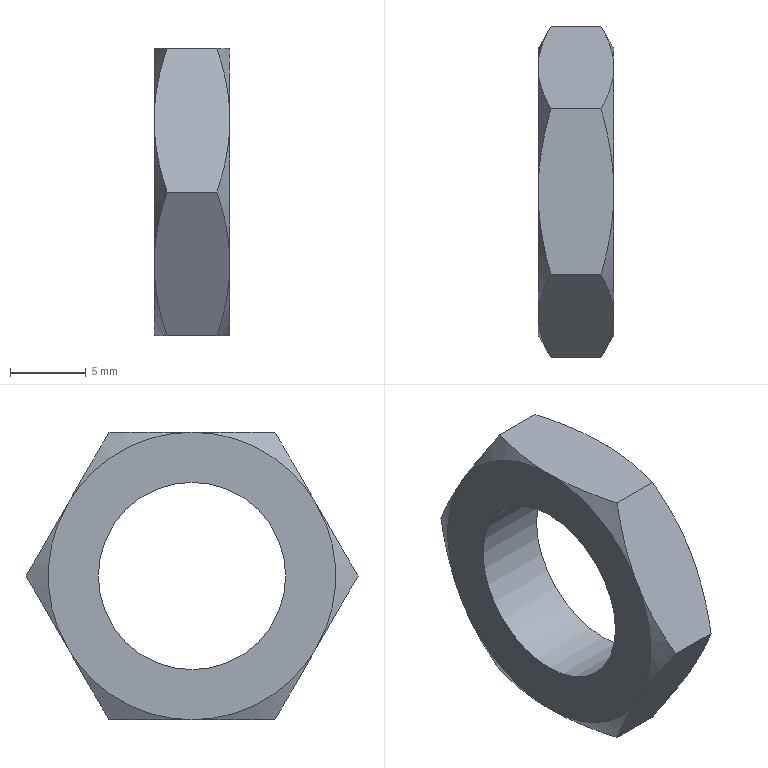Part | NX | features NAT_5003_019_C-AC1412S 2 | 1 solid | 21 faces | box 5 x 21.939 x 19 mm | volume 946.478 mm3 | cone 12 | plane 8 | cylinder 1 | commonest cylinder face diameters 12.376 x1
STEP:
#1=CARTESIAN_POINT('',(56.752,-131.515,-232.5));
#2=VERTEX_POINT('',#1);
#3=CARTESIAN_POINT('',(57.6,-128.773,-227.75));
#4=VERTEX_POINT('',#3);
#5=CARTESIAN_POINT('',(56.752,-131.515,-232.5));
#6=CARTESIAN_POINT('',(57.27,-130.618,-230.946));
#7=CARTESIAN_POINT('',(57.6,-129.707,-229.369));
#8=CARTESIAN_POINT('',(57.6,-128.773,-227.75));
#9=B_SPLINE_CURVE_WITH_KNOTS('',3,(#5,#6,#7,#8),.UNSPECIFIED.,.F.,.F.,(4,4),(0.000000238,0.00555),.UNSPECIFIED.);
#10=EDGE_CURVE('',#2,#4,#9,.T.);
#11=ORIENTED_EDGE('',*,*,#10,.F.);
#12=CARTESIAN_POINT('',(53.449,-131.515,-232.5));
#13=VERTEX_POINT('',#12);
#14=CARTESIAN_POINT('',(57.6,-131.515,-232.5));
#15=DIRECTION('',(-1.,0.,0.));
#16=VECTOR('',#15,1000.);
#17=LINE('',#14,#16);
#18=EDGE_CURVE('',#2,#13,#17,.T.);
#19=ORIENTED_EDGE('',*,*,#18,.T.);
#20=CARTESIAN_POINT('',(52.6,-128.773,-227.75));
#21=VERTEX_POINT('',#20);
#22=CARTESIAN_POINT('',(52.6,-128.773,-227.75));
#23=CARTESIAN_POINT('',(52.6,-129.704,-229.362));
#24=CARTESIAN_POINT('',(52.932,-130.62,-230.95));
#25=CARTESIAN_POINT('',(53.449,-131.515,-232.5));
#26=B_SPLINE_CURVE_WITH_KNOTS('',3,(#22,#23,#24,#25),.UNSPECIFIED.,.F.,.F.,(4,4),(0.00555,0.01108),.UNSPECIFIED.);
#27=EDGE_CURVE('',#21,#13,#26,.T.);
#28=ORIENTED_EDGE('',*,*,#27,.F.);
#29=CARTESIAN_POINT('',(53.449,-126.03,-223.));
#30=VERTEX_POINT('',#29);
#31=CARTESIAN_POINT('',(53.449,-126.03,-223.));
#32=CARTESIAN_POINT('',(52.931,-126.928,-224.554));
#33=CARTESIAN_POINT('',(52.6,-127.838,-226.131));
#34=CARTESIAN_POINT('',(52.6,-128.773,-227.75));
#35=B_SPLINE_CURVE_WITH_KNOTS('',3,(#31,#32,#33,#34),.UNSPECIFIED.,.F.,.F.,(4,4),(0.000000238,0.00555),.UNSPECIFIED.);
#36=EDGE_CURVE('',#30,#21,#35,.T.);
#37=ORIENTED_EDGE('',*,*,#36,.F.);
#38=CARTESIAN_POINT('',(56.752,-126.03,-223.));
#39=VERTEX_POINT('',#38);
#40=CARTESIAN_POINT('',(57.6,-126.03,-223.));
#41=DIRECTION('',(-1.,0.,0.));
#42=VECTOR('',#41,1000.);
#43=LINE('',#40,#42);
#44=EDGE_CURVE('',#39,#30,#43,.T.);
#45=ORIENTED_EDGE('',*,*,#44,.F.);
#46=CARTESIAN_POINT('',(57.6,-128.773,-227.75));
#47=CARTESIAN_POINT('',(57.6,-127.842,-226.138));
#48=CARTESIAN_POINT('',(57.269,-126.925,-224.55));
#49=CARTESIAN_POINT('',(56.752,-126.03,-223.));
#50=B_SPLINE_CURVE_WITH_KNOTS('',3,(#46,#47,#48,#49),.UNSPECIFIED.,.F.,.F.,(4,4),(0.00555,0.01108),.UNSPECIFIED.);
#51=EDGE_CURVE('',#4,#39,#50,.T.);
#52=ORIENTED_EDGE('',*,*,#51,.F.);
#53=EDGE_LOOP('',(#11,#19,#28,#37,#45,#52));
#54=FACE_BOUND('',#53,.T.);
#55=CARTESIAN_POINT('',(57.6,-131.515,-232.5));
#56=DIRECTION('',(0.,-0.866,0.5));
#57=DIRECTION('',(0.,-0.5,-0.866));
#58=AXIS2_PLACEMENT_3D('',#55,#56,#57);
#59=PLANE('',#58);
#60=ADVANCED_FACE('',(#54),#59,.F.);
#61=CARTESIAN_POINT('',(57.6,-128.773,-218.25));
#62=VERTEX_POINT('',#61);
#63=CARTESIAN_POINT('',(56.752,-126.03,-223.));
#64=CARTESIAN_POINT('',(57.27,-126.928,-221.446));
#65=CARTESIAN_POINT('',(57.6,-127.838,-219.869));
#66=CARTESIAN_POINT('',(57.6,-128.773,-218.25));
#67=B_SPLINE_CURVE_WITH_KNOTS('',3,(#63,#64,#65,#66),.UNSPECIFIED.,.F.,.F.,(4,4),(0.000000238,0.00555),.UNSPECIFIED.);
#68=EDGE_CURVE('',#39,#62,#67,.T.);
#69=ORIENTED_EDGE('',*,*,#68,.F.);
#70=ORIENTED_EDGE('',*,*,#44,.T.);
#71=CARTESIAN_POINT('',(52.6,-128.773,-218.25));
#72=VERTEX_POINT('',#71);
#73=CARTESIAN_POINT('',(52.6,-128.773,-218.25));
#74=CARTESIAN_POINT('',(52.6,-127.842,-219.862));
#75=CARTESIAN_POINT('',(52.932,-126.925,-221.45));
#76=CARTESIAN_POINT('',(53.449,-126.03,-223.));
#77=B_SPLINE_CURVE_WITH_KNOTS('',3,(#73,#74,#75,#76),.UNSPECIFIED.,.F.,.F.,(4,4),(0.00555,0.01108),.UNSPECIFIED.);
#78=EDGE_CURVE('',#72,#30,#77,.T.);
#79=ORIENTED_EDGE('',*,*,#78,.F.);
#80=CARTESIAN_POINT('',(53.449,-131.515,-213.5));
#81=VERTEX_POINT('',#80);
#82=CARTESIAN_POINT('',(53.449,-131.515,-213.5));
#83=CARTESIAN_POINT('',(52.931,-130.618,-215.054));
#84=CARTESIAN_POINT('',(52.6,-129.707,-216.631));
#85=CARTESIAN_POINT('',(52.6,-128.773,-218.25));
#86=B_SPLINE_CURVE_WITH_KNOTS('',3,(#82,#83,#84,#85),.UNSPECIFIED.,.F.,.F.,(4,4),(0.000000238,0.00555),.UNSPECIFIED.);
#87=EDGE_CURVE('',#81,#72,#86,.T.);
#88=ORIENTED_EDGE('',*,*,#87,.F.);
#89=CARTESIAN_POINT('',(56.752,-131.515,-213.5));
#90=VERTEX_POINT('',#89);
#91=CARTESIAN_POINT('',(57.6,-131.515,-213.5));
#92=DIRECTION('',(-1.,0.,0.));
#93=VECTOR('',#92,1000.);
#94=LINE('',#91,#93);
#95=EDGE_CURVE('',#90,#81,#94,.T.);
#96=ORIENTED_EDGE('',*,*,#95,.F.);
#97=CARTESIAN_POINT('',(57.6,-128.773,-218.25));
#98=CARTESIAN_POINT('',(57.6,-129.704,-216.638));
#99=CARTESIAN_POINT('',(57.269,-130.62,-215.05));
#100=CARTESIAN_POINT('',(56.752,-131.515,-213.5));
#101=B_SPLINE_CURVE_WITH_KNOTS('',3,(#97,#98,#99,#100),.UNSPECIFIED.,.F.,.F.,(4,4),(0.00555,0.01108),.UNSPECIFIED.);
#102=EDGE_CURVE('',#62,#90,#101,.T.);
#103=ORIENTED_EDGE('',*,*,#102,.F.);
#104=EDGE_LOOP('',(#69,#70,#79,#88,#96,#103));
#105=FACE_BOUND('',#104,.T.);
#106=CARTESIAN_POINT('',(57.6,-126.03,-223.));
#107=DIRECTION('',(0.,-0.866,-0.5));
#108=DIRECTION('',(0.,0.5,-0.866));
#109=AXIS2_PLACEMENT_3D('',#106,#107,#108);
#110=PLANE('',#109);
#111=ADVANCED_FACE('',(#105),#110,.F.);
#112=CARTESIAN_POINT('',(57.6,-137.,-213.5));
#113=VERTEX_POINT('',#112);
#114=CARTESIAN_POINT('',(56.752,-131.515,-213.5));
#115=CARTESIAN_POINT('',(57.267,-133.301,-213.5));
#116=CARTESIAN_POINT('',(57.6,-135.145,-213.5));
#117=CARTESIAN_POINT('',(57.6,-137.,-213.5));
#118=B_SPLINE_CURVE_WITH_KNOTS('',3,(#114,#115,#116,#117),.UNSPECIFIED.,.F.,.F.,(4,4),(0.01001,0.01556),.UNSPECIFIED.);
#119=EDGE_CURVE('',#90,#113,#118,.T.);
#120=ORIENTED_EDGE('',*,*,#119,.F.);
#121=ORIENTED_EDGE('',*,*,#95,.T.);
#122=CARTESIAN_POINT('',(52.6,-137.,-213.5));
#123=VERTEX_POINT('',#122);
#124=CARTESIAN_POINT('',(53.449,-131.515,-213.5));
#125=CARTESIAN_POINT('',(52.934,-133.301,-213.5));
#126=CARTESIAN_POINT('',(52.6,-135.145,-213.5));
#127=CARTESIAN_POINT('',(52.6,-137.,-213.5));
#128=B_SPLINE_CURVE_WITH_KNOTS('',3,(#124,#125,#126,#127),.UNSPECIFIED.,.F.,.F.,(4,4),(0.01001,0.01556),.UNSPECIFIED.);
#129=EDGE_CURVE('',#123,#81,#128,.F.);
#130=ORIENTED_EDGE('',*,*,#129,.F.);
#131=CARTESIAN_POINT('',(53.449,-142.485,-213.5));
#132=VERTEX_POINT('',#131);
#133=CARTESIAN_POINT('',(52.6,-137.,-213.5));
#134=CARTESIAN_POINT('',(52.6,-138.856,-213.5));
#135=CARTESIAN_POINT('',(52.937,-140.711,-213.5));
#136=CARTESIAN_POINT('',(53.449,-142.485,-213.5));
#137=B_SPLINE_CURVE_WITH_KNOTS('',3,(#133,#134,#135,#136),.UNSPECIFIED.,.F.,.F.,(4,4),(0.01556,0.02112),.UNSPECIFIED.);
#138=EDGE_CURVE('',#132,#123,#137,.F.);
#139=ORIENTED_EDGE('',*,*,#138,.F.);
#140=CARTESIAN_POINT('',(56.752,-142.485,-213.5));
#141=VERTEX_POINT('',#140);
#142=CARTESIAN_POINT('',(57.6,-142.485,-213.5));
#143=DIRECTION('',(-1.,0.,0.));
#144=VECTOR('',#143,1000.);
#145=LINE('',#142,#144);
#146=EDGE_CURVE('',#141,#132,#145,.T.);
#147=ORIENTED_EDGE('',*,*,#146,.F.);
#148=CARTESIAN_POINT('',(57.6,-137.,-213.5));
#149=CARTESIAN_POINT('',(57.6,-138.856,-213.5));
#150=CARTESIAN_POINT('',(57.264,-140.711,-213.5));
#151=CARTESIAN_POINT('',(56.752,-142.485,-213.5));
#152=B_SPLINE_CURVE_WITH_KNOTS('',3,(#148,#149,#150,#151),.UNSPECIFIED.,.F.,.F.,(4,4),(0.01556,0.02112),.UNSPECIFIED.);
#153=EDGE_CURVE('',#113,#141,#152,.T.);
#154=ORIENTED_EDGE('',*,*,#153,.F.);
#155=EDGE_LOOP('',(#120,#121,#130,#139,#147,#154));
#156=FACE_BOUND('',#155,.T.);
#157=CARTESIAN_POINT('',(57.6,-131.515,-213.5));
#158=DIRECTION('',(0.,0.,-1.));
#159=DIRECTION('',(0.,1.,0.));
#160=AXIS2_PLACEMENT_3D('',#157,#158,#159);
#161=PLANE('',#160);
#162=ADVANCED_FACE('',(#156),#161,.F.);
#163=CARTESIAN_POINT('',(57.6,-145.227,-218.25));
#164=VERTEX_POINT('',#163);
#165=CARTESIAN_POINT('',(56.752,-142.485,-213.5));
#166=CARTESIAN_POINT('',(57.27,-143.382,-215.054));
#167=CARTESIAN_POINT('',(57.6,-144.293,-216.631));
#168=CARTESIAN_POINT('',(57.6,-145.227,-218.25));
#169=B_SPLINE_CURVE_WITH_KNOTS('',3,(#165,#166,#167,#168),.UNSPECIFIED.,.F.,.F.,(4,4),(0.000000238,0.00555),.UNSPECIFIED.);
#170=EDGE_CURVE('',#141,#164,#169,.T.);
#171=ORIENTED_EDGE('',*,*,#170,.F.);
#172=ORIENTED_EDGE('',*,*,#146,.T.);
#173=CARTESIAN_POINT('',(52.6,-145.227,-218.25));
#174=VERTEX_POINT('',#173);
#175=CARTESIAN_POINT('',(52.6,-145.227,-218.25));
#176=CARTESIAN_POINT('',(52.6,-144.296,-216.638));
#177=CARTESIAN_POINT('',(52.932,-143.38,-215.05));
#178=CARTESIAN_POINT('',(53.449,-142.485,-213.5));
#179=B_SPLINE_CURVE_WITH_KNOTS('',3,(#175,#176,#177,#178),.UNSPECIFIED.,.F.,.F.,(4,4),(0.00555,0.01108),.UNSPECIFIED.);
#180=EDGE_CURVE('',#174,#132,#179,.T.);
#181=ORIENTED_EDGE('',*,*,#180,.F.);
#182=CARTESIAN_POINT('',(53.449,-147.97,-223.));
#183=VERTEX_POINT('',#182);
#184=CARTESIAN_POINT('',(53.449,-147.97,-223.));
#185=CARTESIAN_POINT('',(52.931,-147.072,-221.446));
#186=CARTESIAN_POINT('',(52.6,-146.162,-219.869));
#187=CARTESIAN_POINT('',(52.6,-145.227,-218.25));
#188=B_SPLINE_CURVE_WITH_KNOTS('',3,(#184,#185,#186,#187),.UNSPECIFIED.,.F.,.F.,(4,4),(0.000000238,0.00555),.UNSPECIFIED.);
#189=EDGE_CURVE('',#183,#174,#188,.T.);
#190=ORIENTED_EDGE('',*,*,#189,.F.);
#191=CARTESIAN_POINT('',(56.752,-147.97,-223.));
#192=VERTEX_POINT('',#191);
#193=CARTESIAN_POINT('',(57.6,-147.97,-223.));
#194=DIRECTION('',(-1.,0.,0.));
#195=VECTOR('',#194,1000.);
#196=LINE('',#193,#195);
#197=EDGE_CURVE('',#192,#183,#196,.T.);
#198=ORIENTED_EDGE('',*,*,#197,.F.);
#199=CARTESIAN_POINT('',(57.6,-145.227,-218.25));
#200=CARTESIAN_POINT('',(57.6,-146.158,-219.862));
#201=CARTESIAN_POINT('',(57.269,-147.075,-221.45));
#202=CARTESIAN_POINT('',(56.752,-147.97,-223.));
#203=B_SPLINE_CURVE_WITH_KNOTS('',3,(#199,#200,#201,#202),.UNSPECIFIED.,.F.,.F.,(4,4),(0.00555,0.01108),.UNSPECIFIED.);
#204=EDGE_CURVE('',#164,#192,#203,.T.);
#205=ORIENTED_EDGE('',*,*,#204,.F.);
#206=EDGE_LOOP('',(#171,#172,#181,#190,#198,#205));
#207=FACE_BOUND('',#206,.T.);
#208=CARTESIAN_POINT('',(57.6,-142.485,-213.5));
#209=DIRECTION('',(0.,0.866,-0.5));
#210=DIRECTION('',(0.,0.5,0.866));
#211=AXIS2_PLACEMENT_3D('',#208,#209,#210);
#212=PLANE('',#211);
#213=ADVANCED_FACE('',(#207),#212,.F.);
#214=CARTESIAN_POINT('',(57.6,-145.227,-227.75));
#215=VERTEX_POINT('',#214);
#216=CARTESIAN_POINT('',(56.752,-147.97,-223.));
#217=CARTESIAN_POINT('',(57.27,-147.072,-224.554));
#218=CARTESIAN_POINT('',(57.6,-146.162,-226.131));
#219=CARTESIAN_POINT('',(57.6,-145.227,-227.75));
#220=B_SPLINE_CURVE_WITH_KNOTS('',3,(#216,#217,#218,#219),.UNSPECIFIED.,.F.,.F.,(4,4),(0.000000238,0.00555),.UNSPECIFIED.);
#221=EDGE_CURVE('',#192,#215,#220,.T.);
#222=ORIENTED_EDGE('',*,*,#221,.F.);
#223=ORIENTED_EDGE('',*,*,#197,.T.);
#224=CARTESIAN_POINT('',(52.6,-145.227,-227.75));
#225=VERTEX_POINT('',#224);
#226=CARTESIAN_POINT('',(52.6,-145.227,-227.75));
#227=CARTESIAN_POINT('',(52.6,-146.158,-226.138));
#228=CARTESIAN_POINT('',(52.932,-147.075,-224.55));
#229=CARTESIAN_POINT('',(53.449,-147.97,-223.));
#230=B_SPLINE_CURVE_WITH_KNOTS('',3,(#226,#227,#228,#229),.UNSPECIFIED.,.F.,.F.,(4,4),(0.00555,0.01108),.UNSPECIFIED.);
#231=EDGE_CURVE('',#225,#183,#230,.T.);
#232=ORIENTED_EDGE('',*,*,#231,.F.);
#233=CARTESIAN_POINT('',(53.449,-142.485,-232.5));
#234=VERTEX_POINT('',#233);
#235=CARTESIAN_POINT('',(53.449,-142.485,-232.5));
#236=CARTESIAN_POINT('',(52.931,-143.382,-230.946));
#237=CARTESIAN_POINT('',(52.6,-144.293,-229.369));
#238=CARTESIAN_POINT('',(52.6,-145.227,-227.75));
#239=B_SPLINE_CURVE_WITH_KNOTS('',3,(#235,#236,#237,#238),.UNSPECIFIED.,.F.,.F.,(4,4),(0.000000238,0.00555),.UNSPECIFIED.);
#240=EDGE_CURVE('',#234,#225,#239,.T.);
#241=ORIENTED_EDGE('',*,*,#240,.F.);
#242=CARTESIAN_POINT('',(56.752,-142.485,-232.5));
#243=VERTEX_POINT('',#242);
#244=CARTESIAN_POINT('',(57.6,-142.485,-232.5));
#245=DIRECTION('',(-1.,0.,0.));
#246=VECTOR('',#245,1000.);
#247=LINE('',#244,#246);
#248=EDGE_CURVE('',#243,#234,#247,.T.);
#249=ORIENTED_EDGE('',*,*,#248,.F.);
#250=CARTESIAN_POINT('',(57.6,-145.227,-227.75));
#251=CARTESIAN_POINT('',(57.6,-144.296,-229.362));
#252=CARTESIAN_POINT('',(57.269,-143.38,-230.95));
#253=CARTESIAN_POINT('',(56.752,-142.485,-232.5));
#254=B_SPLINE_CURVE_WITH_KNOTS('',3,(#250,#251,#252,#253),.UNSPECIFIED.,.F.,.F.,(4,4),(0.00555,0.01108),.UNSPECIFIED.);
#255=EDGE_CURVE('',#215,#243,#254,.T.);
#256=ORIENTED_EDGE('',*,*,#255,.F.);
#257=EDGE_LOOP('',(#222,#223,#232,#241,#249,#256));
#258=FACE_BOUND('',#257,.T.);
#259=CARTESIAN_POINT('',(57.6,-147.97,-223.));
#260=DIRECTION('',(0.,0.866,0.5));
#261=DIRECTION('',(0.,-0.5,0.866));
#262=AXIS2_PLACEMENT_3D('',#259,#260,#261);
#263=PLANE('',#262);
#264=ADVANCED_FACE('',(#258),#263,.F.);
#265=CARTESIAN_POINT('',(57.6,-137.,-232.5));
#266=VERTEX_POINT('',#265);
#267=CARTESIAN_POINT('',(57.6,-137.,-232.5));
#268=CARTESIAN_POINT('',(57.6,-138.856,-232.5));
#269=CARTESIAN_POINT('',(57.264,-140.711,-232.5));
#270=CARTESIAN_POINT('',(56.752,-142.485,-232.5));
#271=B_SPLINE_CURVE_WITH_KNOTS('',3,(#267,#268,#269,#270),.UNSPECIFIED.,.F.,.F.,(4,4),(0.01556,0.02112),.UNSPECIFIED.);
#272=EDGE_CURVE('',#243,#266,#271,.F.);
#273=ORIENTED_EDGE('',*,*,#272,.F.);
#274=ORIENTED_EDGE('',*,*,#248,.T.);
#275=CARTESIAN_POINT('',(52.6,-137.,-232.5));
#276=VERTEX_POINT('',#275);
#277=CARTESIAN_POINT('',(52.6,-137.,-232.5));
#278=CARTESIAN_POINT('',(52.6,-138.856,-232.5));
#279=CARTESIAN_POINT('',(52.937,-140.711,-232.5));
#280=CARTESIAN_POINT('',(53.449,-142.485,-232.5));
#281=B_SPLINE_CURVE_WITH_KNOTS('',3,(#277,#278,#279,#280),.UNSPECIFIED.,.F.,.F.,(4,4),(0.01556,0.02112),.UNSPECIFIED.);
#282=EDGE_CURVE('',#276,#234,#281,.T.);
#283=ORIENTED_EDGE('',*,*,#282,.F.);
#284=CARTESIAN_POINT('',(53.449,-131.515,-232.5));
#285=CARTESIAN_POINT('',(52.934,-133.301,-232.5));
#286=CARTESIAN_POINT('',(52.6,-135.145,-232.5));
#287=CARTESIAN_POINT('',(52.6,-137.,-232.5));
#288=B_SPLINE_CURVE_WITH_KNOTS('',3,(#284,#285,#286,#287),.UNSPECIFIED.,.F.,.F.,(4,4),(0.01001,0.01556),.UNSPECIFIED.);
#289=EDGE_CURVE('',#13,#276,#288,.T.);
#290=ORIENTED_EDGE('',*,*,#289,.F.);
#291=ORIENTED_EDGE('',*,*,#18,.F.);
#292=CARTESIAN_POINT('',(56.752,-131.515,-232.5));
#293=CARTESIAN_POINT('',(57.267,-133.301,-232.5));
#294=CARTESIAN_POINT('',(57.6,-135.145,-232.5));
#295=CARTESIAN_POINT('',(57.6,-137.,-232.5));
#296=B_SPLINE_CURVE_WITH_KNOTS('',3,(#292,#293,#294,#295),.UNSPECIFIED.,.F.,.F.,(4,4),(0.01001,0.01556),.UNSPECIFIED.);
#297=EDGE_CURVE('',#266,#2,#296,.F.);
#298=ORIENTED_EDGE('',*,*,#297,.F.);
#299=EDGE_LOOP('',(#273,#274,#283,#290,#291,#298));
#300=FACE_BOUND('',#299,.T.);
#301=CARTESIAN_POINT('',(57.6,-142.485,-232.5));
#302=DIRECTION('',(0.,0.,1.));
#303=DIRECTION('',(0.,-1.,0.));
#304=AXIS2_PLACEMENT_3D('',#301,#302,#303);
#305=PLANE('',#304);
#306=ADVANCED_FACE('',(#300),#305,.F.);
#307=CARTESIAN_POINT('',(57.6,-130.812,-223.));
#308=VERTEX_POINT('',#307);
#309=CARTESIAN_POINT('',(57.6,-137.,-223.));
#310=DIRECTION('',(1.,0.,0.));
#311=DIRECTION('',(0.,1.,0.));
#312=AXIS2_PLACEMENT_3D('',#309,#310,#311);
#313=CIRCLE('',#312,6.188);
#314=EDGE_CURVE('',#308,#308,#313,.T.);
#315=ORIENTED_EDGE('',*,*,#314,.F.);
#316=EDGE_LOOP('',(#315));
#317=FACE_BOUND('',#316,.T.);
#318=CARTESIAN_POINT('',(57.6,-137.,-223.));
#319=DIRECTION('',(1.,0.,0.));
#320=DIRECTION('',(0.,1.,0.));
#321=AXIS2_PLACEMENT_3D('',#318,#319,#320);
#322=CIRCLE('',#321,9.5);
#323=EDGE_CURVE('',#4,#62,#322,.T.);
#324=ORIENTED_EDGE('',*,*,#323,.T.);
#325=CARTESIAN_POINT('',(57.6,-137.,-223.));
#326=DIRECTION('',(1.,0.,0.));
#327=DIRECTION('',(0.,1.,0.));
#328=AXIS2_PLACEMENT_3D('',#325,#326,#327);
#329=CIRCLE('',#328,9.5);
#330=EDGE_CURVE('',#62,#113,#329,.T.);
#331=ORIENTED_EDGE('',*,*,#330,.T.);
#332=CARTESIAN_POINT('',(57.6,-137.,-223.));
#333=DIRECTION('',(-1.,0.,0.));
#334=DIRECTION('',(0.,-1.,0.));
#335=AXIS2_PLACEMENT_3D('',#332,#333,#334);
#336=CIRCLE('',#335,9.5);
#337=EDGE_CURVE('',#164,#113,#336,.T.);
#338=ORIENTED_EDGE('',*,*,#337,.F.);
#339=CARTESIAN_POINT('',(57.6,-137.,-223.));
#340=DIRECTION('',(1.,0.,0.));
#341=DIRECTION('',(0.,1.,0.));
#342=AXIS2_PLACEMENT_3D('',#339,#340,#341);
#343=CIRCLE('',#342,9.5);
#344=EDGE_CURVE('',#164,#215,#343,.T.);
#345=ORIENTED_EDGE('',*,*,#344,.T.);
#346=CARTESIAN_POINT('',(57.6,-137.,-223.));
#347=DIRECTION('',(1.,0.,0.));
#348=DIRECTION('',(0.,1.,0.));
#349=AXIS2_PLACEMENT_3D('',#346,#347,#348);
#350=CIRCLE('',#349,9.5);
#351=EDGE_CURVE('',#215,#266,#350,.T.);
#352=ORIENTED_EDGE('',*,*,#351,.T.);
#353=CARTESIAN_POINT('',(57.6,-137.,-223.));
#354=DIRECTION('',(1.,0.,0.));
#355=DIRECTION('',(0.,1.,0.));
#356=AXIS2_PLACEMENT_3D('',#353,#354,#355);
#357=CIRCLE('',#356,9.5);
#358=EDGE_CURVE('',#266,#4,#357,.T.);
#359=ORIENTED_EDGE('',*,*,#358,.T.);
#360=EDGE_LOOP('',(#324,#331,#338,#345,#352,#359));
#361=FACE_BOUND('',#360,.T.);
#362=CARTESIAN_POINT('',(57.6,-137.,-223.));
#363=DIRECTION('',(1.,0.,0.));
#364=DIRECTION('',(0.,1.,0.));
#365=AXIS2_PLACEMENT_3D('',#362,#363,#364);
#366=PLANE('',#365);
#367=ADVANCED_FACE('',(#317,#361),#366,.T.);
#368=CARTESIAN_POINT('',(52.6,-130.812,-223.));
#369=VERTEX_POINT('',#368);
#370=CARTESIAN_POINT('',(52.6,-137.,-223.));
#371=DIRECTION('',(1.,0.,0.));
#372=DIRECTION('',(0.,1.,0.));
#373=AXIS2_PLACEMENT_3D('',#370,#371,#372);
#374=CIRCLE('',#373,6.188);
#375=EDGE_CURVE('',#369,#369,#374,.T.);
#376=ORIENTED_EDGE('',*,*,#375,.T.);
#377=EDGE_LOOP('',(#376));
#378=FACE_BOUND('',#377,.T.);
#379=CARTESIAN_POINT('',(52.6,-137.,-223.));
#380=DIRECTION('',(1.,0.,0.));
#381=DIRECTION('',(0.,1.,0.));
#382=AXIS2_PLACEMENT_3D('',#379,#380,#381);
#383=CIRCLE('',#382,9.5);
#384=EDGE_CURVE('',#72,#123,#383,.T.);
#385=ORIENTED_EDGE('',*,*,#384,.F.);
#386=CARTESIAN_POINT('',(52.6,-137.,-223.));
#387=DIRECTION('',(1.,0.,0.));
#388=DIRECTION('',(0.,1.,0.));
#389=AXIS2_PLACEMENT_3D('',#386,#387,#388);
#390=CIRCLE('',#389,9.5);
#391=EDGE_CURVE('',#21,#72,#390,.T.);
#392=ORIENTED_EDGE('',*,*,#391,.F.);
#393=CARTESIAN_POINT('',(52.6,-137.,-223.));
#394=DIRECTION('',(1.,0.,0.));
#395=DIRECTION('',(0.,1.,0.));
#396=AXIS2_PLACEMENT_3D('',#393,#394,#395);
#397=CIRCLE('',#396,9.5);
#398=EDGE_CURVE('',#276,#21,#397,.T.);
#399=ORIENTED_EDGE('',*,*,#398,.F.);
#400=CARTESIAN_POINT('',(52.6,-137.,-223.));
#401=DIRECTION('',(1.,0.,0.));
#402=DIRECTION('',(0.,1.,0.));
#403=AXIS2_PLACEMENT_3D('',#400,#401,#402);
#404=CIRCLE('',#403,9.5);
#405=EDGE_CURVE('',#225,#276,#404,.T.);
#406=ORIENTED_EDGE('',*,*,#405,.F.);
#407=CARTESIAN_POINT('',(52.6,-137.,-223.));
#408=DIRECTION('',(1.,0.,0.));
#409=DIRECTION('',(0.,1.,0.));
#410=AXIS2_PLACEMENT_3D('',#407,#408,#409);
#411=CIRCLE('',#410,9.5);
#412=EDGE_CURVE('',#174,#225,#411,.T.);
#413=ORIENTED_EDGE('',*,*,#412,.F.);
#414=CARTESIAN_POINT('',(52.6,-137.,-223.));
#415=DIRECTION('',(-1.,0.,0.));
#416=DIRECTION('',(0.,-1.,0.));
#417=AXIS2_PLACEMENT_3D('',#414,#415,#416);
#418=CIRCLE('',#417,9.5);
#419=EDGE_CURVE('',#174,#123,#418,.T.);
#420=ORIENTED_EDGE('',*,*,#419,.T.);
#421=EDGE_LOOP('',(#385,#392,#399,#406,#413,#420));
#422=FACE_BOUND('',#421,.T.);
#423=CARTESIAN_POINT('',(52.6,-137.,-223.));
#424=DIRECTION('',(1.,0.,0.));
#425=DIRECTION('',(0.,1.,0.));
#426=AXIS2_PLACEMENT_3D('',#423,#424,#425);
#427=PLANE('',#426);
#428=ADVANCED_FACE('',(#378,#422),#427,.F.);
#429=ORIENTED_EDGE('',*,*,#375,.F.);
#430=EDGE_LOOP('',(#429));
#431=FACE_BOUND('',#430,.T.);
#432=ORIENTED_EDGE('',*,*,#314,.T.);
#433=EDGE_LOOP('',(#432));
#434=FACE_BOUND('',#433,.T.);
#435=CARTESIAN_POINT('',(57.6,-137.,-223.));
#436=DIRECTION('',(1.,0.,0.));
#437=DIRECTION('',(0.,1.,0.));
#438=AXIS2_PLACEMENT_3D('',#435,#436,#437);
#439=CYLINDRICAL_SURFACE('',#438,6.188);
#440=ADVANCED_FACE('',(#431,#434),#439,.F.);
#441=ORIENTED_EDGE('',*,*,#78,.T.);
#442=ORIENTED_EDGE('',*,*,#36,.T.);
#443=ORIENTED_EDGE('',*,*,#391,.T.);
#444=EDGE_LOOP('',(#441,#442,#443));
#445=FACE_BOUND('',#444,.T.);
#446=CARTESIAN_POINT('',(52.6,-137.,-223.));
#447=DIRECTION('',(1.,0.,0.));
#448=DIRECTION('',(0.,1.,0.));
#449=AXIS2_PLACEMENT_3D('',#446,#447,#448);
#450=CONICAL_SURFACE('',#449,9.5,1.047);
#451=ADVANCED_FACE('',(#445),#450,.T.);
#452=ORIENTED_EDGE('',*,*,#27,.T.);
#453=ORIENTED_EDGE('',*,*,#289,.T.);
#454=ORIENTED_EDGE('',*,*,#398,.T.);
#455=EDGE_LOOP('',(#452,#453,#454));
#456=FACE_BOUND('',#455,.T.);
#457=CARTESIAN_POINT('',(52.6,-137.,-223.));
#458=DIRECTION('',(1.,0.,0.));
#459=DIRECTION('',(0.,1.,0.));
#460=AXIS2_PLACEMENT_3D('',#457,#458,#459);
#461=CONICAL_SURFACE('',#460,9.5,1.047);
#462=ADVANCED_FACE('',(#456),#461,.T.);
#463=ORIENTED_EDGE('',*,*,#240,.T.);
#464=ORIENTED_EDGE('',*,*,#405,.T.);
#465=ORIENTED_EDGE('',*,*,#282,.T.);
#466=EDGE_LOOP('',(#463,#464,#465));
#467=FACE_BOUND('',#466,.T.);
#468=CARTESIAN_POINT('',(52.6,-137.,-223.));
#469=DIRECTION('',(1.,0.,0.));
#470=DIRECTION('',(0.,1.,0.));
#471=AXIS2_PLACEMENT_3D('',#468,#469,#470);
#472=CONICAL_SURFACE('',#471,9.5,1.047);
#473=ADVANCED_FACE('',(#467),#472,.T.);
#474=ORIENTED_EDGE('',*,*,#189,.T.);
#475=ORIENTED_EDGE('',*,*,#412,.T.);
#476=ORIENTED_EDGE('',*,*,#231,.T.);
#477=EDGE_LOOP('',(#474,#475,#476));
#478=FACE_BOUND('',#477,.T.);
#479=CARTESIAN_POINT('',(52.6,-137.,-223.));
#480=DIRECTION('',(1.,0.,0.));
#481=DIRECTION('',(0.,1.,0.));
#482=AXIS2_PLACEMENT_3D('',#479,#480,#481);
#483=CONICAL_SURFACE('',#482,9.5,1.047);
#484=ADVANCED_FACE('',(#478),#483,.T.);
#485=ORIENTED_EDGE('',*,*,#138,.T.);
#486=ORIENTED_EDGE('',*,*,#419,.F.);
#487=ORIENTED_EDGE('',*,*,#180,.T.);
#488=EDGE_LOOP('',(#485,#486,#487));
#489=FACE_BOUND('',#488,.T.);
#490=CARTESIAN_POINT('',(52.6,-137.,-223.));
#491=DIRECTION('',(1.,0.,0.));
#492=DIRECTION('',(0.,1.,0.));
#493=AXIS2_PLACEMENT_3D('',#490,#491,#492);
#494=CONICAL_SURFACE('',#493,9.5,1.047);
#495=ADVANCED_FACE('',(#489),#494,.T.);
#496=ORIENTED_EDGE('',*,*,#129,.T.);
#497=ORIENTED_EDGE('',*,*,#87,.T.);
#498=ORIENTED_EDGE('',*,*,#384,.T.);
#499=EDGE_LOOP('',(#496,#497,#498));
#500=FACE_BOUND('',#499,.T.);
#501=CARTESIAN_POINT('',(52.6,-137.,-223.));
#502=DIRECTION('',(1.,0.,0.));
#503=DIRECTION('',(0.,1.,0.));
#504=AXIS2_PLACEMENT_3D('',#501,#502,#503);
#505=CONICAL_SURFACE('',#504,9.5,1.047);
#506=ADVANCED_FACE('',(#500),#505,.T.);
#507=ORIENTED_EDGE('',*,*,#51,.T.);
#508=ORIENTED_EDGE('',*,*,#68,.T.);
#509=ORIENTED_EDGE('',*,*,#323,.F.);
#510=EDGE_LOOP('',(#507,#508,#509));
#511=FACE_BOUND('',#510,.T.);
#512=CARTESIAN_POINT('',(55.291,-137.,-223.));
#513=DIRECTION('',(-1.,0.,0.));
#514=DIRECTION('',(0.,-1.,0.));
#515=AXIS2_PLACEMENT_3D('',#512,#513,#514);
#516=CONICAL_SURFACE('',#515,13.5,1.047);
#517=ADVANCED_FACE('',(#511),#516,.T.);
#518=ORIENTED_EDGE('',*,*,#10,.T.);
#519=ORIENTED_EDGE('',*,*,#358,.F.);
#520=ORIENTED_EDGE('',*,*,#297,.T.);
#521=EDGE_LOOP('',(#518,#519,#520));
#522=FACE_BOUND('',#521,.T.);
#523=CARTESIAN_POINT('',(55.291,-137.,-223.));
#524=DIRECTION('',(-1.,0.,0.));
#525=DIRECTION('',(0.,-1.,0.));
#526=AXIS2_PLACEMENT_3D('',#523,#524,#525);
#527=CONICAL_SURFACE('',#526,13.5,1.047);
#528=ADVANCED_FACE('',(#522),#527,.T.);
#529=ORIENTED_EDGE('',*,*,#255,.T.);
#530=ORIENTED_EDGE('',*,*,#272,.T.);
#531=ORIENTED_EDGE('',*,*,#351,.F.);
#532=EDGE_LOOP('',(#529,#530,#531));
#533=FACE_BOUND('',#532,.T.);
#534=CARTESIAN_POINT('',(55.291,-137.,-223.));
#535=DIRECTION('',(-1.,0.,0.));
#536=DIRECTION('',(0.,-1.,0.));
#537=AXIS2_PLACEMENT_3D('',#534,#535,#536);
#538=CONICAL_SURFACE('',#537,13.5,1.047);
#539=ADVANCED_FACE('',(#533),#538,.T.);
#540=ORIENTED_EDGE('',*,*,#204,.T.);
#541=ORIENTED_EDGE('',*,*,#221,.T.);
#542=ORIENTED_EDGE('',*,*,#344,.F.);
#543=EDGE_LOOP('',(#540,#541,#542));
#544=FACE_BOUND('',#543,.T.);
#545=CARTESIAN_POINT('',(55.291,-137.,-223.));
#546=DIRECTION('',(-1.,0.,0.));
#547=DIRECTION('',(0.,-1.,0.));
#548=AXIS2_PLACEMENT_3D('',#545,#546,#547);
#549=CONICAL_SURFACE('',#548,13.5,1.047);
#550=ADVANCED_FACE('',(#544),#549,.T.);
#551=ORIENTED_EDGE('',*,*,#153,.T.);
#552=ORIENTED_EDGE('',*,*,#170,.T.);
#553=ORIENTED_EDGE('',*,*,#337,.T.);
#554=EDGE_LOOP('',(#551,#552,#553));
#555=FACE_BOUND('',#554,.T.);
#556=CARTESIAN_POINT('',(55.291,-137.,-223.));
#557=DIRECTION('',(-1.,0.,0.));
#558=DIRECTION('',(0.,-1.,0.));
#559=AXIS2_PLACEMENT_3D('',#556,#557,#558);
#560=CONICAL_SURFACE('',#559,13.5,1.047);
#561=ADVANCED_FACE('',(#555),#560,.T.);
#562=ORIENTED_EDGE('',*,*,#102,.T.);
#563=ORIENTED_EDGE('',*,*,#119,.T.);
#564=ORIENTED_EDGE('',*,*,#330,.F.);
#565=EDGE_LOOP('',(#562,#563,#564));
#566=FACE_BOUND('',#565,.T.);
#567=CARTESIAN_POINT('',(55.291,-137.,-223.));
#568=DIRECTION('',(-1.,0.,0.));
#569=DIRECTION('',(0.,-1.,0.));
#570=AXIS2_PLACEMENT_3D('',#567,#568,#569);
#571=CONICAL_SURFACE('',#570,13.5,1.047);
#572=ADVANCED_FACE('',(#566),#571,.T.);
#573=CLOSED_SHELL('',(#60,#111,#162,#213,#264,#306,#367,#428,#440,#451,#462,#473,#484,#495,#506,#517,#528,#539,#550,#561,#572));
#574=MANIFOLD_SOLID_BREP('',#573);
#575=(LENGTH_UNIT()NAMED_UNIT(*)SI_UNIT(.MILLI.,.METRE.));
#576=UNCERTAINTY_MEASURE_WITH_UNIT(LENGTH_MEASURE(0.0508),#575,'','');
#577=(NAMED_UNIT(*)PLANE_ANGLE_UNIT()SI_UNIT($,.RADIAN.));
#578=(NAMED_UNIT(*)SI_UNIT($,.STERADIAN.)SOLID_ANGLE_UNIT());
#579=(GEOMETRIC_REPRESENTATION_CONTEXT(3)GLOBAL_UNCERTAINTY_ASSIGNED_CONTEXT((#576))GLOBAL_UNIT_ASSIGNED_CONTEXT((#575,#577,#578))REPRESENTATION_CONTEXT('',''));
#580=ADVANCED_BREP_SHAPE_REPRESENTATION('',(#574),#579);